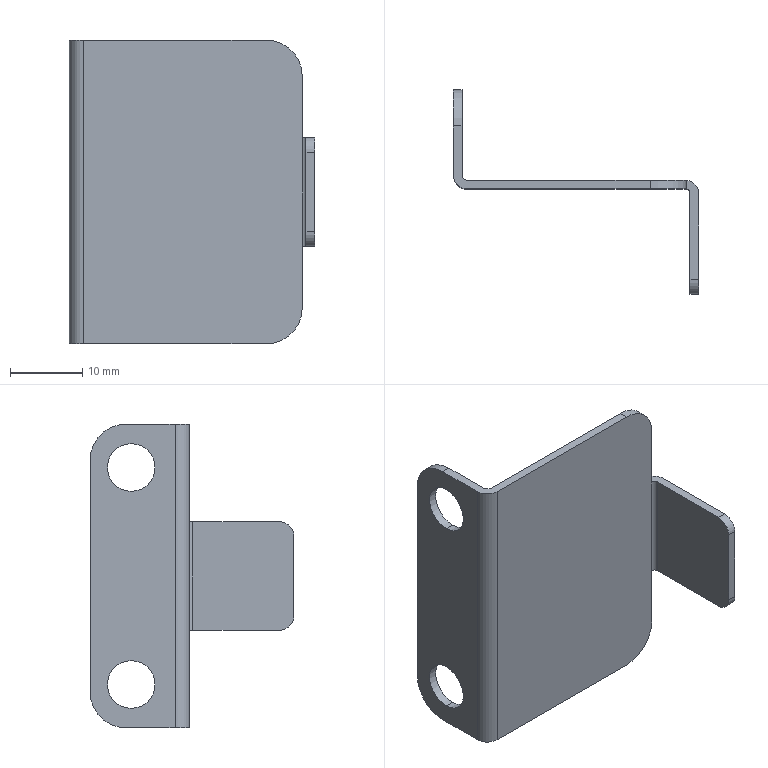Part | SolidWorks | features BaseBody 1 | 1 solid | 28 faces | box 33.9 x 28.2 x 42 mm | volume 2397 mm3 | cylinder 14 | plane 14 | commonest cylinder face diameters 6.6 x4 10 x4 4 x2 1 x1 1.473 x1 3.4 x1
STEP:
#1=CARTESIAN_POINT('',(0.,6.8,0.7));
#2=VERTEX_POINT('',#1);
#3=CARTESIAN_POINT('',(0.,6.8,7.3));
#4=VERTEX_POINT('',#3);
#5=CARTESIAN_POINT('',(0.,6.8,4.));
#6=DIRECTION('',(-1.,0.,0.));
#7=DIRECTION('',(0.,0.,1.));
#8=AXIS2_PLACEMENT_3D('',#5,#6,#7);
#9=CIRCLE('',#8,3.3);
#10=EDGE_CURVE('',#2,#4,#9,.T.);
#11=ORIENTED_EDGE('',*,*,#10,.F.);
#12=CARTESIAN_POINT('',(-1.2,6.8,0.7));
#13=VERTEX_POINT('',#12);
#14=CARTESIAN_POINT('',(-1.2,6.8,0.7));
#15=DIRECTION('',(-1.,0.,0.));
#16=VECTOR('',#15,1000.);
#17=LINE('',#14,#16);
#18=EDGE_CURVE('',#2,#13,#17,.T.);
#19=ORIENTED_EDGE('',*,*,#18,.T.);
#20=CARTESIAN_POINT('',(-1.2,6.8,7.3));
#21=VERTEX_POINT('',#20);
#22=CARTESIAN_POINT('',(-1.2,6.8,4.));
#23=DIRECTION('',(-1.,0.,0.));
#24=DIRECTION('',(0.,0.,1.));
#25=AXIS2_PLACEMENT_3D('',#22,#23,#24);
#26=CIRCLE('',#25,3.3);
#27=EDGE_CURVE('',#13,#21,#26,.T.);
#28=ORIENTED_EDGE('',*,*,#27,.T.);
#29=CARTESIAN_POINT('',(-1.2,6.8,7.3));
#30=DIRECTION('',(-1.,0.,0.));
#31=VECTOR('',#30,1000.);
#32=LINE('',#29,#31);
#33=EDGE_CURVE('',#4,#21,#32,.T.);
#34=ORIENTED_EDGE('',*,*,#33,.F.);
#35=EDGE_LOOP('',(#11,#19,#28,#34));
#36=FACE_OUTER_BOUND('',#35,.T.);
#37=CARTESIAN_POINT('',(-1.2,6.8,4.));
#38=DIRECTION('',(-1.,0.,0.));
#39=DIRECTION('',(0.,0.,1.));
#40=AXIS2_PLACEMENT_3D('',#37,#38,#39);
#41=CYLINDRICAL_SURFACE('',#40,3.3);
#42=ADVANCED_FACE('',(#36),#41,.F.);
#43=CARTESIAN_POINT('',(0.,6.8,-29.3));
#44=VERTEX_POINT('',#43);
#45=CARTESIAN_POINT('',(0.,6.8,-22.7));
#46=VERTEX_POINT('',#45);
#47=CARTESIAN_POINT('',(0.,6.8,-26.));
#48=DIRECTION('',(-1.,0.,0.));
#49=DIRECTION('',(0.,0.,1.));
#50=AXIS2_PLACEMENT_3D('',#47,#48,#49);
#51=CIRCLE('',#50,3.3);
#52=EDGE_CURVE('',#44,#46,#51,.T.);
#53=ORIENTED_EDGE('',*,*,#52,.F.);
#54=CARTESIAN_POINT('',(-1.2,6.8,-29.3));
#55=VERTEX_POINT('',#54);
#56=CARTESIAN_POINT('',(-1.2,6.8,-29.3));
#57=DIRECTION('',(-1.,0.,0.));
#58=VECTOR('',#57,1000.);
#59=LINE('',#56,#58);
#60=EDGE_CURVE('',#44,#55,#59,.T.);
#61=ORIENTED_EDGE('',*,*,#60,.T.);
#62=CARTESIAN_POINT('',(-1.2,6.8,-22.7));
#63=VERTEX_POINT('',#62);
#64=CARTESIAN_POINT('',(-1.2,6.8,-26.));
#65=DIRECTION('',(-1.,0.,0.));
#66=DIRECTION('',(0.,0.,1.));
#67=AXIS2_PLACEMENT_3D('',#64,#65,#66);
#68=CIRCLE('',#67,3.3);
#69=EDGE_CURVE('',#55,#63,#68,.T.);
#70=ORIENTED_EDGE('',*,*,#69,.T.);
#71=CARTESIAN_POINT('',(-1.2,6.8,-22.7));
#72=DIRECTION('',(-1.,0.,0.));
#73=VECTOR('',#72,1000.);
#74=LINE('',#71,#73);
#75=EDGE_CURVE('',#46,#63,#74,.T.);
#76=ORIENTED_EDGE('',*,*,#75,.F.);
#77=EDGE_LOOP('',(#53,#61,#70,#76));
#78=FACE_OUTER_BOUND('',#77,.T.);
#79=CARTESIAN_POINT('',(-1.2,6.8,-26.));
#80=DIRECTION('',(-1.,0.,0.));
#81=DIRECTION('',(0.,0.,1.));
#82=AXIS2_PLACEMENT_3D('',#79,#80,#81);
#83=CYLINDRICAL_SURFACE('',#82,3.3);
#84=ADVANCED_FACE('',(#78),#83,.F.);
#85=CARTESIAN_POINT('',(26.,-1.2,10.));
#86=VERTEX_POINT('',#85);
#87=CARTESIAN_POINT('',(31.,-1.2,5.));
#88=VERTEX_POINT('',#87);
#89=CARTESIAN_POINT('',(26.,-1.2,5.));
#90=DIRECTION('',(0.,1.,0.));
#91=DIRECTION('',(0.,0.,-1.));
#92=AXIS2_PLACEMENT_3D('',#89,#90,#91);
#93=CIRCLE('',#92,5.);
#94=EDGE_CURVE('',#86,#88,#93,.T.);
#95=ORIENTED_EDGE('',*,*,#94,.F.);
#96=CARTESIAN_POINT('',(0.7366,-1.2,10.));
#97=VERTEX_POINT('',#96);
#98=CARTESIAN_POINT('',(0.,-1.2,10.));
#99=DIRECTION('',(1.,0.,0.));
#100=VECTOR('',#99,1000.);
#101=LINE('',#98,#100);
#102=EDGE_CURVE('',#97,#86,#101,.T.);
#103=ORIENTED_EDGE('',*,*,#102,.F.);
#104=CARTESIAN_POINT('',(0.7366,-1.2,-32.));
#105=VERTEX_POINT('',#104);
#106=CARTESIAN_POINT('',(0.7366,-1.2,10.));
#107=DIRECTION('',(0.,0.,1.));
#108=VECTOR('',#107,1000.);
#109=LINE('',#106,#108);
#110=EDGE_CURVE('',#105,#97,#109,.T.);
#111=ORIENTED_EDGE('',*,*,#110,.F.);
#112=CARTESIAN_POINT('',(26.,-1.2,-32.));
#113=VERTEX_POINT('',#112);
#114=CARTESIAN_POINT('',(0.,-1.2,-32.));
#115=DIRECTION('',(-1.,0.,0.));
#116=VECTOR('',#115,1000.);
#117=LINE('',#114,#116);
#118=EDGE_CURVE('',#113,#105,#117,.T.);
#119=ORIENTED_EDGE('',*,*,#118,.F.);
#120=CARTESIAN_POINT('',(31.,-1.2,-27.));
#121=VERTEX_POINT('',#120);
#122=CARTESIAN_POINT('',(26.,-1.2,-27.));
#123=DIRECTION('',(0.,1.,0.));
#124=DIRECTION('',(0.,0.,-1.));
#125=AXIS2_PLACEMENT_3D('',#122,#123,#124);
#126=CIRCLE('',#125,5.);
#127=EDGE_CURVE('',#121,#113,#126,.T.);
#128=ORIENTED_EDGE('',*,*,#127,.F.);
#129=CARTESIAN_POINT('',(31.,-1.2,-18.5));
#130=VERTEX_POINT('',#129);
#131=CARTESIAN_POINT('',(31.,-1.2,10.));
#132=DIRECTION('',(0.,0.,-1.));
#133=VECTOR('',#132,1000.);
#134=LINE('',#131,#133);
#135=EDGE_CURVE('',#130,#121,#134,.T.);
#136=ORIENTED_EDGE('',*,*,#135,.F.);
#137=CARTESIAN_POINT('',(31.,-1.2,-3.5));
#138=VERTEX_POINT('',#137);
#139=CARTESIAN_POINT('',(31.,-1.2,10.));
#140=DIRECTION('',(0.,0.,-1.));
#141=VECTOR('',#140,1000.);
#142=LINE('',#139,#141);
#143=EDGE_CURVE('',#138,#130,#142,.T.);
#144=ORIENTED_EDGE('',*,*,#143,.F.);
#145=CARTESIAN_POINT('',(31.,-1.2,10.));
#146=DIRECTION('',(0.,0.,-1.));
#147=VECTOR('',#146,1000.);
#148=LINE('',#145,#147);
#149=EDGE_CURVE('',#88,#138,#148,.T.);
#150=ORIENTED_EDGE('',*,*,#149,.F.);
#151=EDGE_LOOP('',(#95,#103,#111,#119,#128,#136,#144,#150));
#152=FACE_OUTER_BOUND('',#151,.T.);
#153=CARTESIAN_POINT('',(0.,-1.2,10.));
#154=DIRECTION('',(0.,1.,0.));
#155=DIRECTION('',(0.,0.,1.));
#156=AXIS2_PLACEMENT_3D('',#153,#154,#155);
#157=PLANE('',#156);
#158=ADVANCED_FACE('',(#152),#157,.F.);
#159=ORIENTED_EDGE('',*,*,#149,.T.);
#160=CARTESIAN_POINT('',(31.,0.,-3.5));
#161=VERTEX_POINT('',#160);
#162=CARTESIAN_POINT('',(31.,-1.7,-3.5));
#163=DIRECTION('',(0.,1.,0.));
#164=VECTOR('',#163,1000.);
#165=LINE('',#162,#164);
#166=EDGE_CURVE('',#138,#161,#165,.T.);
#167=ORIENTED_EDGE('',*,*,#166,.T.);
#168=CARTESIAN_POINT('',(31.,0.,5.));
#169=VERTEX_POINT('',#168);
#170=CARTESIAN_POINT('',(31.,0.,10.));
#171=DIRECTION('',(0.,0.,1.));
#172=VECTOR('',#171,1000.);
#173=LINE('',#170,#172);
#174=EDGE_CURVE('',#161,#169,#173,.T.);
#175=ORIENTED_EDGE('',*,*,#174,.T.);
#176=CARTESIAN_POINT('',(31.,0.,5.));
#177=DIRECTION('',(0.,-1.,0.));
#178=VECTOR('',#177,1000.);
#179=LINE('',#176,#178);
#180=EDGE_CURVE('',#169,#88,#179,.T.);
#181=ORIENTED_EDGE('',*,*,#180,.T.);
#182=EDGE_LOOP('',(#159,#167,#175,#181));
#183=FACE_OUTER_BOUND('',#182,.T.);
#184=CARTESIAN_POINT('',(31.,0.,10.));
#185=DIRECTION('',(1.,0.,0.));
#186=DIRECTION('',(0.,0.,-1.));
#187=AXIS2_PLACEMENT_3D('',#184,#185,#186);
#188=PLANE('',#187);
#189=ADVANCED_FACE('',(#183),#188,.T.);
#190=ORIENTED_EDGE('',*,*,#94,.T.);
#191=ORIENTED_EDGE('',*,*,#180,.F.);
#192=CARTESIAN_POINT('',(26.,0.,10.));
#193=VERTEX_POINT('',#192);
#194=CARTESIAN_POINT('',(26.,0.,5.));
#195=DIRECTION('',(0.,-1.,0.));
#196=DIRECTION('',(0.,0.,-1.));
#197=AXIS2_PLACEMENT_3D('',#194,#195,#196);
#198=CIRCLE('',#197,5.);
#199=EDGE_CURVE('',#169,#193,#198,.T.);
#200=ORIENTED_EDGE('',*,*,#199,.T.);
#201=CARTESIAN_POINT('',(26.,0.,10.));
#202=DIRECTION('',(0.,-1.,0.));
#203=VECTOR('',#202,1000.);
#204=LINE('',#201,#203);
#205=EDGE_CURVE('',#193,#86,#204,.T.);
#206=ORIENTED_EDGE('',*,*,#205,.T.);
#207=EDGE_LOOP('',(#190,#191,#200,#206));
#208=FACE_OUTER_BOUND('',#207,.T.);
#209=CARTESIAN_POINT('',(26.,0.,5.));
#210=DIRECTION('',(0.,-1.,0.));
#211=DIRECTION('',(0.,0.,-1.));
#212=AXIS2_PLACEMENT_3D('',#209,#210,#211);
#213=CYLINDRICAL_SURFACE('',#212,5.);
#214=ADVANCED_FACE('',(#208),#213,.T.);
#215=CARTESIAN_POINT('',(0.7366,0.,10.));
#216=VERTEX_POINT('',#215);
#217=CARTESIAN_POINT('',(-1.2,0.,10.));
#218=DIRECTION('',(-1.,0.,0.));
#219=VECTOR('',#218,1000.);
#220=LINE('',#217,#219);
#221=EDGE_CURVE('',#193,#216,#220,.T.);
#222=ORIENTED_EDGE('',*,*,#221,.T.);
#223=CARTESIAN_POINT('',(0.,0.7366,10.));
#224=VERTEX_POINT('',#223);
#225=CARTESIAN_POINT('',(0.7366,0.7366,10.));
#226=DIRECTION('',(0.,0.,-1.));
#227=DIRECTION('',(-1.,0.,0.));
#228=AXIS2_PLACEMENT_3D('',#225,#226,#227);
#229=CIRCLE('',#228,0.7366);
#230=EDGE_CURVE('',#216,#224,#229,.T.);
#231=ORIENTED_EDGE('',*,*,#230,.T.);
#232=CARTESIAN_POINT('',(0.,7.5,10.));
#233=VERTEX_POINT('',#232);
#234=CARTESIAN_POINT('',(0.,0.7366,10.));
#235=DIRECTION('',(0.,-1.,0.));
#236=VECTOR('',#235,1000.);
#237=LINE('',#234,#236);
#238=EDGE_CURVE('',#233,#224,#237,.T.);
#239=ORIENTED_EDGE('',*,*,#238,.F.);
#240=CARTESIAN_POINT('',(-1.2,7.5,10.));
#241=VERTEX_POINT('',#240);
#242=CARTESIAN_POINT('',(0.7366,7.5,10.));
#243=DIRECTION('',(1.,0.,0.));
#244=VECTOR('',#243,1000.);
#245=LINE('',#242,#244);
#246=EDGE_CURVE('',#241,#233,#245,.T.);
#247=ORIENTED_EDGE('',*,*,#246,.F.);
#248=CARTESIAN_POINT('',(-1.2,0.7366,10.));
#249=VERTEX_POINT('',#248);
#250=CARTESIAN_POINT('',(-1.2,12.5,10.));
#251=DIRECTION('',(0.,-1.,0.));
#252=VECTOR('',#251,1000.);
#253=LINE('',#250,#252);
#254=EDGE_CURVE('',#241,#249,#253,.T.);
#255=ORIENTED_EDGE('',*,*,#254,.T.);
#256=CARTESIAN_POINT('',(0.7366,0.7366,10.));
#257=DIRECTION('',(0.,0.,-1.));
#258=DIRECTION('',(-1.,0.,0.));
#259=AXIS2_PLACEMENT_3D('',#256,#257,#258);
#260=CIRCLE('',#259,1.937);
#261=EDGE_CURVE('',#97,#249,#260,.T.);
#262=ORIENTED_EDGE('',*,*,#261,.F.);
#263=ORIENTED_EDGE('',*,*,#102,.T.);
#264=ORIENTED_EDGE('',*,*,#205,.F.);
#265=EDGE_LOOP('',(#222,#231,#239,#247,#255,#262,#263,#264));
#266=FACE_OUTER_BOUND('',#265,.T.);
#267=CARTESIAN_POINT('',(-1.2,0.7366,10.));
#268=DIRECTION('',(0.,0.,1.));
#269=DIRECTION('',(1.,0.,0.));
#270=AXIS2_PLACEMENT_3D('',#267,#268,#269);
#271=PLANE('',#270);
#272=ADVANCED_FACE('',(#266),#271,.T.);
#273=ORIENTED_EDGE('',*,*,#110,.T.);
#274=ORIENTED_EDGE('',*,*,#261,.T.);
#275=CARTESIAN_POINT('',(-1.2,0.7366,-32.));
#276=VERTEX_POINT('',#275);
#277=CARTESIAN_POINT('',(-1.2,0.7366,10.));
#278=DIRECTION('',(0.,0.,-1.));
#279=VECTOR('',#278,1000.);
#280=LINE('',#277,#279);
#281=EDGE_CURVE('',#249,#276,#280,.T.);
#282=ORIENTED_EDGE('',*,*,#281,.T.);
#283=CARTESIAN_POINT('',(0.7366,0.7366,-32.));
#284=DIRECTION('',(0.,0.,1.));
#285=DIRECTION('',(-1.,0.,0.));
#286=AXIS2_PLACEMENT_3D('',#283,#284,#285);
#287=CIRCLE('',#286,1.937);
#288=EDGE_CURVE('',#276,#105,#287,.T.);
#289=ORIENTED_EDGE('',*,*,#288,.T.);
#290=EDGE_LOOP('',(#273,#274,#282,#289));
#291=FACE_OUTER_BOUND('',#290,.T.);
#292=CARTESIAN_POINT('',(0.7366,0.7366,10.));
#293=DIRECTION('',(0.,0.,-1.));
#294=DIRECTION('',(-1.,0.,0.));
#295=AXIS2_PLACEMENT_3D('',#292,#293,#294);
#296=CYLINDRICAL_SURFACE('',#295,1.937);
#297=ADVANCED_FACE('',(#291),#296,.T.);
#298=ORIENTED_EDGE('',*,*,#118,.T.);
#299=ORIENTED_EDGE('',*,*,#288,.F.);
#300=CARTESIAN_POINT('',(-1.2,7.5,-32.));
#301=VERTEX_POINT('',#300);
#302=CARTESIAN_POINT('',(-1.2,12.5,-32.));
#303=DIRECTION('',(0.,1.,0.));
#304=VECTOR('',#303,1000.);
#305=LINE('',#302,#304);
#306=EDGE_CURVE('',#276,#301,#305,.T.);
#307=ORIENTED_EDGE('',*,*,#306,.T.);
#308=CARTESIAN_POINT('',(0.,7.5,-32.));
#309=VERTEX_POINT('',#308);
#310=CARTESIAN_POINT('',(0.7366,7.5,-32.));
#311=DIRECTION('',(-1.,0.,0.));
#312=VECTOR('',#311,1000.);
#313=LINE('',#310,#312);
#314=EDGE_CURVE('',#309,#301,#313,.T.);
#315=ORIENTED_EDGE('',*,*,#314,.F.);
#316=CARTESIAN_POINT('',(0.,0.7366,-32.));
#317=VERTEX_POINT('',#316);
#318=CARTESIAN_POINT('',(0.,-1.2,-32.));
#319=DIRECTION('',(0.,-1.,0.));
#320=VECTOR('',#319,1000.);
#321=LINE('',#318,#320);
#322=EDGE_CURVE('',#309,#317,#321,.T.);
#323=ORIENTED_EDGE('',*,*,#322,.T.);
#324=CARTESIAN_POINT('',(0.7366,0.,-32.));
#325=VERTEX_POINT('',#324);
#326=CARTESIAN_POINT('',(0.7366,0.7366,-32.));
#327=DIRECTION('',(0.,0.,1.));
#328=DIRECTION('',(-1.,0.,0.));
#329=AXIS2_PLACEMENT_3D('',#326,#327,#328);
#330=CIRCLE('',#329,0.7366);
#331=EDGE_CURVE('',#317,#325,#330,.T.);
#332=ORIENTED_EDGE('',*,*,#331,.T.);
#333=CARTESIAN_POINT('',(26.,0.,-32.));
#334=VERTEX_POINT('',#333);
#335=CARTESIAN_POINT('',(0.7366,0.,-32.));
#336=DIRECTION('',(1.,0.,0.));
#337=VECTOR('',#336,1000.);
#338=LINE('',#335,#337);
#339=EDGE_CURVE('',#325,#334,#338,.T.);
#340=ORIENTED_EDGE('',*,*,#339,.T.);
#341=CARTESIAN_POINT('',(26.,0.7366,-32.));
#342=DIRECTION('',(0.,-1.,0.));
#343=VECTOR('',#342,1000.);
#344=LINE('',#341,#343);
#345=EDGE_CURVE('',#334,#113,#344,.T.);
#346=ORIENTED_EDGE('',*,*,#345,.T.);
#347=EDGE_LOOP('',(#298,#299,#307,#315,#323,#332,#340,#346));
#348=FACE_OUTER_BOUND('',#347,.T.);
#349=CARTESIAN_POINT('',(0.7366,0.7366,-32.));
#350=DIRECTION('',(0.,0.,-1.));
#351=DIRECTION('',(-1.,0.,0.));
#352=AXIS2_PLACEMENT_3D('',#349,#350,#351);
#353=PLANE('',#352);
#354=ADVANCED_FACE('',(#348),#353,.T.);
#355=ORIENTED_EDGE('',*,*,#127,.T.);
#356=ORIENTED_EDGE('',*,*,#345,.F.);
#357=CARTESIAN_POINT('',(31.,0.,-27.));
#358=VERTEX_POINT('',#357);
#359=CARTESIAN_POINT('',(26.,0.,-27.));
#360=DIRECTION('',(0.,-1.,0.));
#361=DIRECTION('',(0.,0.,-1.));
#362=AXIS2_PLACEMENT_3D('',#359,#360,#361);
#363=CIRCLE('',#362,5.);
#364=EDGE_CURVE('',#334,#358,#363,.T.);
#365=ORIENTED_EDGE('',*,*,#364,.T.);
#366=CARTESIAN_POINT('',(31.,0.7366,-27.));
#367=DIRECTION('',(0.,-1.,0.));
#368=VECTOR('',#367,1000.);
#369=LINE('',#366,#368);
#370=EDGE_CURVE('',#358,#121,#369,.T.);
#371=ORIENTED_EDGE('',*,*,#370,.T.);
#372=EDGE_LOOP('',(#355,#356,#365,#371));
#373=FACE_OUTER_BOUND('',#372,.T.);
#374=CARTESIAN_POINT('',(26.,0.7366,-27.));
#375=DIRECTION('',(0.,-1.,0.));
#376=DIRECTION('',(0.,0.,-1.));
#377=AXIS2_PLACEMENT_3D('',#374,#375,#376);
#378=CYLINDRICAL_SURFACE('',#377,5.);
#379=ADVANCED_FACE('',(#373),#378,.T.);
#380=CARTESIAN_POINT('',(31.,0.,-18.5));
#381=VERTEX_POINT('',#380);
#382=CARTESIAN_POINT('',(31.,0.,10.));
#383=DIRECTION('',(0.,0.,1.));
#384=VECTOR('',#383,1000.);
#385=LINE('',#382,#384);
#386=EDGE_CURVE('',#358,#381,#385,.T.);
#387=ORIENTED_EDGE('',*,*,#386,.T.);
#388=CARTESIAN_POINT('',(31.,-1.7,-18.5));
#389=DIRECTION('',(0.,1.,0.));
#390=VECTOR('',#389,1000.);
#391=LINE('',#388,#390);
#392=EDGE_CURVE('',#130,#381,#391,.T.);
#393=ORIENTED_EDGE('',*,*,#392,.F.);
#394=ORIENTED_EDGE('',*,*,#135,.T.);
#395=ORIENTED_EDGE('',*,*,#370,.F.);
#396=EDGE_LOOP('',(#387,#393,#394,#395));
#397=FACE_OUTER_BOUND('',#396,.T.);
#398=CARTESIAN_POINT('',(31.,0.,10.));
#399=DIRECTION('',(1.,0.,0.));
#400=DIRECTION('',(0.,0.,-1.));
#401=AXIS2_PLACEMENT_3D('',#398,#399,#400);
#402=PLANE('',#401);
#403=ADVANCED_FACE('',(#397),#402,.T.);
#404=CARTESIAN_POINT('',(31.5,-1.7,-18.5));
#405=VERTEX_POINT('',#404);
#406=CARTESIAN_POINT('',(31.,-1.7,-18.5));
#407=DIRECTION('',(0.,0.,1.));
#408=DIRECTION('',(1.,0.,0.));
#409=AXIS2_PLACEMENT_3D('',#406,#407,#408);
#410=CIRCLE('',#409,0.5);
#411=EDGE_CURVE('',#405,#130,#410,.T.);
#412=ORIENTED_EDGE('',*,*,#411,.F.);
#413=CARTESIAN_POINT('',(31.5,-1.7,-3.5));
#414=VERTEX_POINT('',#413);
#415=CARTESIAN_POINT('',(31.5,-1.7,-3.5));
#416=DIRECTION('',(0.,0.,-1.));
#417=VECTOR('',#416,1000.);
#418=LINE('',#415,#417);
#419=EDGE_CURVE('',#414,#405,#418,.T.);
#420=ORIENTED_EDGE('',*,*,#419,.F.);
#421=CARTESIAN_POINT('',(31.,-1.7,-3.5));
#422=DIRECTION('',(0.,0.,1.));
#423=DIRECTION('',(1.,0.,0.));
#424=AXIS2_PLACEMENT_3D('',#421,#422,#423);
#425=CIRCLE('',#424,0.5);
#426=EDGE_CURVE('',#414,#138,#425,.T.);
#427=ORIENTED_EDGE('',*,*,#426,.T.);
#428=ORIENTED_EDGE('',*,*,#143,.T.);
#429=EDGE_LOOP('',(#412,#420,#427,#428));
#430=FACE_OUTER_BOUND('',#429,.T.);
#431=CARTESIAN_POINT('',(31.,-1.7,-3.5));
#432=DIRECTION('',(0.,0.,1.));
#433=DIRECTION('',(1.,0.,0.));
#434=AXIS2_PLACEMENT_3D('',#431,#432,#433);
#435=CYLINDRICAL_SURFACE('',#434,0.5);
#436=ADVANCED_FACE('',(#430),#435,.F.);
#437=ORIENTED_EDGE('',*,*,#339,.F.);
#438=CARTESIAN_POINT('',(0.7366,0.,10.));
#439=DIRECTION('',(0.,0.,1.));
#440=VECTOR('',#439,1000.);
#441=LINE('',#438,#440);
#442=EDGE_CURVE('',#325,#216,#441,.T.);
#443=ORIENTED_EDGE('',*,*,#442,.T.);
#444=ORIENTED_EDGE('',*,*,#221,.F.);
#445=ORIENTED_EDGE('',*,*,#199,.F.);
#446=ORIENTED_EDGE('',*,*,#174,.F.);
#447=CARTESIAN_POINT('',(31.,0.,10.));
#448=DIRECTION('',(0.,0.,-1.));
#449=VECTOR('',#448,1000.);
#450=LINE('',#447,#449);
#451=EDGE_CURVE('',#161,#381,#450,.T.);
#452=ORIENTED_EDGE('',*,*,#451,.T.);
#453=ORIENTED_EDGE('',*,*,#386,.F.);
#454=ORIENTED_EDGE('',*,*,#364,.F.);
#455=EDGE_LOOP('',(#437,#443,#444,#445,#446,#452,#453,#454));
#456=FACE_OUTER_BOUND('',#455,.T.);
#457=CARTESIAN_POINT('',(0.,0.,10.));
#458=DIRECTION('',(0.,1.,0.));
#459=DIRECTION('',(0.,0.,1.));
#460=AXIS2_PLACEMENT_3D('',#457,#458,#459);
#461=PLANE('',#460);
#462=ADVANCED_FACE('',(#456),#461,.T.);
#463=CARTESIAN_POINT('',(-1.2,12.5,5.));
#464=VERTEX_POINT('',#463);
#465=CARTESIAN_POINT('',(-1.2,7.5,5.));
#466=DIRECTION('',(1.,0.,0.));
#467=DIRECTION('',(0.,0.,1.));
#468=AXIS2_PLACEMENT_3D('',#465,#466,#467);
#469=CIRCLE('',#468,5.);
#470=EDGE_CURVE('',#464,#241,#469,.T.);
#471=ORIENTED_EDGE('',*,*,#470,.F.);
#472=CARTESIAN_POINT('',(-1.2,12.5,-27.));
#473=VERTEX_POINT('',#472);
#474=CARTESIAN_POINT('',(-1.2,12.5,10.));
#475=DIRECTION('',(0.,0.,1.));
#476=VECTOR('',#475,1000.);
#477=LINE('',#474,#476);
#478=EDGE_CURVE('',#473,#464,#477,.T.);
#479=ORIENTED_EDGE('',*,*,#478,.F.);
#480=CARTESIAN_POINT('',(-1.2,7.5,-27.));
#481=DIRECTION('',(1.,0.,0.));
#482=DIRECTION('',(0.,0.,-1.));
#483=AXIS2_PLACEMENT_3D('',#480,#481,#482);
#484=CIRCLE('',#483,5.);
#485=EDGE_CURVE('',#301,#473,#484,.T.);
#486=ORIENTED_EDGE('',*,*,#485,.F.);
#487=ORIENTED_EDGE('',*,*,#306,.F.);
#488=ORIENTED_EDGE('',*,*,#281,.F.);
#489=ORIENTED_EDGE('',*,*,#254,.F.);
#490=EDGE_LOOP('',(#471,#479,#486,#487,#488,#489));
#491=FACE_OUTER_BOUND('',#490,.T.);
#492=CARTESIAN_POINT('',(-1.2,6.8,4.));
#493=DIRECTION('',(-1.,0.,0.));
#494=DIRECTION('',(0.,0.,1.));
#495=AXIS2_PLACEMENT_3D('',#492,#493,#494);
#496=CIRCLE('',#495,3.3);
#497=EDGE_CURVE('',#21,#13,#496,.T.);
#498=ORIENTED_EDGE('',*,*,#497,.F.);
#499=ORIENTED_EDGE('',*,*,#27,.F.);
#500=EDGE_LOOP('',(#498,#499));
#501=FACE_BOUND('',#500,.T.);
#502=CARTESIAN_POINT('',(-1.2,6.8,-26.));
#503=DIRECTION('',(-1.,0.,0.));
#504=DIRECTION('',(0.,0.,1.));
#505=AXIS2_PLACEMENT_3D('',#502,#503,#504);
#506=CIRCLE('',#505,3.3);
#507=EDGE_CURVE('',#63,#55,#506,.T.);
#508=ORIENTED_EDGE('',*,*,#507,.F.);
#509=ORIENTED_EDGE('',*,*,#69,.F.);
#510=EDGE_LOOP('',(#508,#509));
#511=FACE_BOUND('',#510,.T.);
#512=CARTESIAN_POINT('',(-1.2,12.5,10.));
#513=DIRECTION('',(1.,0.,0.));
#514=DIRECTION('',(0.,1.,0.));
#515=AXIS2_PLACEMENT_3D('',#512,#513,#514);
#516=PLANE('',#515);
#517=ADVANCED_FACE('',(#491,#501,#511),#516,.F.);
#518=CARTESIAN_POINT('',(31.5,-13.7,-18.5));
#519=VERTEX_POINT('',#518);
#520=CARTESIAN_POINT('',(31.5,0.,-18.5));
#521=DIRECTION('',(0.,-1.,0.));
#522=VECTOR('',#521,1000.);
#523=LINE('',#520,#522);
#524=EDGE_CURVE('',#405,#519,#523,.T.);
#525=ORIENTED_EDGE('',*,*,#524,.T.);
#526=CARTESIAN_POINT('',(31.5,-15.7,-16.5));
#527=VERTEX_POINT('',#526);
#528=CARTESIAN_POINT('',(31.5,-13.7,-16.5));
#529=DIRECTION('',(-1.,0.,0.));
#530=DIRECTION('',(0.,-1.,0.));
#531=AXIS2_PLACEMENT_3D('',#528,#529,#530);
#532=CIRCLE('',#531,2.);
#533=EDGE_CURVE('',#519,#527,#532,.T.);
#534=ORIENTED_EDGE('',*,*,#533,.T.);
#535=CARTESIAN_POINT('',(31.5,-15.7,-5.5));
#536=VERTEX_POINT('',#535);
#537=CARTESIAN_POINT('',(31.5,-15.7,0.));
#538=DIRECTION('',(0.,0.,1.));
#539=VECTOR('',#538,1000.);
#540=LINE('',#537,#539);
#541=EDGE_CURVE('',#527,#536,#540,.T.);
#542=ORIENTED_EDGE('',*,*,#541,.T.);
#543=CARTESIAN_POINT('',(31.5,-13.7,-3.5));
#544=VERTEX_POINT('',#543);
#545=CARTESIAN_POINT('',(31.5,-13.7,-5.5));
#546=DIRECTION('',(-1.,0.,0.));
#547=DIRECTION('',(0.,-1.,0.));
#548=AXIS2_PLACEMENT_3D('',#545,#546,#547);
#549=CIRCLE('',#548,2.);
#550=EDGE_CURVE('',#536,#544,#549,.T.);
#551=ORIENTED_EDGE('',*,*,#550,.T.);
#552=CARTESIAN_POINT('',(31.5,0.,-3.5));
#553=DIRECTION('',(0.,1.,0.));
#554=VECTOR('',#553,1000.);
#555=LINE('',#552,#554);
#556=EDGE_CURVE('',#544,#414,#555,.T.);
#557=ORIENTED_EDGE('',*,*,#556,.T.);
#558=ORIENTED_EDGE('',*,*,#419,.T.);
#559=EDGE_LOOP('',(#525,#534,#542,#551,#557,#558));
#560=FACE_OUTER_BOUND('',#559,.T.);
#561=CARTESIAN_POINT('',(31.5,0.,0.));
#562=DIRECTION('',(-1.,0.,0.));
#563=DIRECTION('',(0.,-1.,0.));
#564=AXIS2_PLACEMENT_3D('',#561,#562,#563);
#565=PLANE('',#564);
#566=ADVANCED_FACE('',(#560),#565,.T.);
#567=ORIENTED_EDGE('',*,*,#331,.F.);
#568=CARTESIAN_POINT('',(0.,0.7366,10.));
#569=DIRECTION('',(0.,0.,-1.));
#570=VECTOR('',#569,1000.);
#571=LINE('',#568,#570);
#572=EDGE_CURVE('',#224,#317,#571,.T.);
#573=ORIENTED_EDGE('',*,*,#572,.F.);
#574=ORIENTED_EDGE('',*,*,#230,.F.);
#575=ORIENTED_EDGE('',*,*,#442,.F.);
#576=EDGE_LOOP('',(#567,#573,#574,#575));
#577=FACE_OUTER_BOUND('',#576,.T.);
#578=CARTESIAN_POINT('',(0.7366,0.7366,10.));
#579=DIRECTION('',(0.,0.,-1.));
#580=DIRECTION('',(-1.,0.,0.));
#581=AXIS2_PLACEMENT_3D('',#578,#579,#580);
#582=CYLINDRICAL_SURFACE('',#581,0.7366);
#583=ADVANCED_FACE('',(#577),#582,.F.);
#584=CARTESIAN_POINT('',(32.7,-1.7,-3.5));
#585=VERTEX_POINT('',#584);
#586=CARTESIAN_POINT('',(32.7,-1.7,-18.5));
#587=VERTEX_POINT('',#586);
#588=CARTESIAN_POINT('',(32.7,-1.7,-3.5));
#589=DIRECTION('',(0.,0.,-1.));
#590=VECTOR('',#589,1000.);
#591=LINE('',#588,#590);
#592=EDGE_CURVE('',#585,#587,#591,.T.);
#593=ORIENTED_EDGE('',*,*,#592,.T.);
#594=CARTESIAN_POINT('',(31.,-1.7,-18.5));
#595=DIRECTION('',(0.,0.,1.));
#596=DIRECTION('',(1.,0.,0.));
#597=AXIS2_PLACEMENT_3D('',#594,#595,#596);
#598=CIRCLE('',#597,1.7);
#599=EDGE_CURVE('',#587,#381,#598,.T.);
#600=ORIENTED_EDGE('',*,*,#599,.T.);
#601=ORIENTED_EDGE('',*,*,#451,.F.);
#602=CARTESIAN_POINT('',(31.,-1.7,-3.5));
#603=DIRECTION('',(0.,0.,-1.));
#604=DIRECTION('',(1.,0.,0.));
#605=AXIS2_PLACEMENT_3D('',#602,#603,#604);
#606=CIRCLE('',#605,1.7);
#607=EDGE_CURVE('',#161,#585,#606,.T.);
#608=ORIENTED_EDGE('',*,*,#607,.T.);
#609=EDGE_LOOP('',(#593,#600,#601,#608));
#610=FACE_OUTER_BOUND('',#609,.T.);
#611=CARTESIAN_POINT('',(31.,-1.7,-3.5));
#612=DIRECTION('',(0.,0.,1.));
#613=DIRECTION('',(1.,0.,0.));
#614=AXIS2_PLACEMENT_3D('',#611,#612,#613);
#615=CYLINDRICAL_SURFACE('',#614,1.7);
#616=ADVANCED_FACE('',(#610),#615,.T.);
#617=CARTESIAN_POINT('',(0.,12.5,5.));
#618=VERTEX_POINT('',#617);
#619=CARTESIAN_POINT('',(0.,7.5,5.));
#620=DIRECTION('',(-1.,0.,0.));
#621=DIRECTION('',(0.,0.,1.));
#622=AXIS2_PLACEMENT_3D('',#619,#620,#621);
#623=CIRCLE('',#622,5.);
#624=EDGE_CURVE('',#233,#618,#623,.T.);
#625=ORIENTED_EDGE('',*,*,#624,.T.);
#626=CARTESIAN_POINT('',(-1.2,12.5,5.));
#627=DIRECTION('',(-1.,0.,0.));
#628=VECTOR('',#627,1000.);
#629=LINE('',#626,#628);
#630=EDGE_CURVE('',#618,#464,#629,.T.);
#631=ORIENTED_EDGE('',*,*,#630,.T.);
#632=ORIENTED_EDGE('',*,*,#470,.T.);
#633=ORIENTED_EDGE('',*,*,#246,.T.);
#634=EDGE_LOOP('',(#625,#631,#632,#633));
#635=FACE_OUTER_BOUND('',#634,.T.);
#636=CARTESIAN_POINT('',(-1.2,7.5,5.));
#637=DIRECTION('',(-1.,0.,0.));
#638=DIRECTION('',(0.,0.,1.));
#639=AXIS2_PLACEMENT_3D('',#636,#637,#638);
#640=CYLINDRICAL_SURFACE('',#639,5.);
#641=ADVANCED_FACE('',(#635),#640,.T.);
#642=CARTESIAN_POINT('',(0.,12.5,-27.));
#643=VERTEX_POINT('',#642);
#644=CARTESIAN_POINT('',(0.,12.5,10.));
#645=DIRECTION('',(0.,0.,-1.));
#646=VECTOR('',#645,1000.);
#647=LINE('',#644,#646);
#648=EDGE_CURVE('',#618,#643,#647,.T.);
#649=ORIENTED_EDGE('',*,*,#648,.T.);
#650=CARTESIAN_POINT('',(-1.2,12.5,-27.));
#651=DIRECTION('',(-1.,0.,0.));
#652=VECTOR('',#651,1000.);
#653=LINE('',#650,#652);
#654=EDGE_CURVE('',#643,#473,#653,.T.);
#655=ORIENTED_EDGE('',*,*,#654,.T.);
#656=ORIENTED_EDGE('',*,*,#478,.T.);
#657=ORIENTED_EDGE('',*,*,#630,.F.);
#658=EDGE_LOOP('',(#649,#655,#656,#657));
#659=FACE_OUTER_BOUND('',#658,.T.);
#660=CARTESIAN_POINT('',(-1.2,12.5,10.));
#661=DIRECTION('',(0.,1.,0.));
#662=DIRECTION('',(0.,0.,1.));
#663=AXIS2_PLACEMENT_3D('',#660,#661,#662);
#664=PLANE('',#663);
#665=ADVANCED_FACE('',(#659),#664,.T.);
#666=CARTESIAN_POINT('',(0.,7.5,-27.));
#667=DIRECTION('',(-1.,0.,0.));
#668=DIRECTION('',(0.,0.,-1.));
#669=AXIS2_PLACEMENT_3D('',#666,#667,#668);
#670=CIRCLE('',#669,5.);
#671=EDGE_CURVE('',#643,#309,#670,.T.);
#672=ORIENTED_EDGE('',*,*,#671,.T.);
#673=ORIENTED_EDGE('',*,*,#314,.T.);
#674=ORIENTED_EDGE('',*,*,#485,.T.);
#675=ORIENTED_EDGE('',*,*,#654,.F.);
#676=EDGE_LOOP('',(#672,#673,#674,#675));
#677=FACE_OUTER_BOUND('',#676,.T.);
#678=CARTESIAN_POINT('',(0.7366,7.5,-27.));
#679=DIRECTION('',(1.,0.,0.));
#680=DIRECTION('',(0.,0.,-1.));
#681=AXIS2_PLACEMENT_3D('',#678,#679,#680);
#682=CYLINDRICAL_SURFACE('',#681,5.);
#683=ADVANCED_FACE('',(#677),#682,.T.);
#684=ORIENTED_EDGE('',*,*,#18,.F.);
#685=CARTESIAN_POINT('',(0.,6.8,4.));
#686=DIRECTION('',(-1.,0.,0.));
#687=DIRECTION('',(0.,0.,1.));
#688=AXIS2_PLACEMENT_3D('',#685,#686,#687);
#689=CIRCLE('',#688,3.3);
#690=EDGE_CURVE('',#4,#2,#689,.T.);
#691=ORIENTED_EDGE('',*,*,#690,.F.);
#692=ORIENTED_EDGE('',*,*,#33,.T.);
#693=ORIENTED_EDGE('',*,*,#497,.T.);
#694=EDGE_LOOP('',(#684,#691,#692,#693));
#695=FACE_OUTER_BOUND('',#694,.T.);
#696=CARTESIAN_POINT('',(-1.2,6.8,4.));
#697=DIRECTION('',(-1.,0.,0.));
#698=DIRECTION('',(0.,0.,1.));
#699=AXIS2_PLACEMENT_3D('',#696,#697,#698);
#700=CYLINDRICAL_SURFACE('',#699,3.3);
#701=ADVANCED_FACE('',(#695),#700,.F.);
#702=ORIENTED_EDGE('',*,*,#60,.F.);
#703=CARTESIAN_POINT('',(0.,6.8,-26.));
#704=DIRECTION('',(-1.,0.,0.));
#705=DIRECTION('',(0.,0.,1.));
#706=AXIS2_PLACEMENT_3D('',#703,#704,#705);
#707=CIRCLE('',#706,3.3);
#708=EDGE_CURVE('',#46,#44,#707,.T.);
#709=ORIENTED_EDGE('',*,*,#708,.F.);
#710=ORIENTED_EDGE('',*,*,#75,.T.);
#711=ORIENTED_EDGE('',*,*,#507,.T.);
#712=EDGE_LOOP('',(#702,#709,#710,#711));
#713=FACE_OUTER_BOUND('',#712,.T.);
#714=CARTESIAN_POINT('',(-1.2,6.8,-26.));
#715=DIRECTION('',(-1.,0.,0.));
#716=DIRECTION('',(0.,0.,1.));
#717=AXIS2_PLACEMENT_3D('',#714,#715,#716);
#718=CYLINDRICAL_SURFACE('',#717,3.3);
#719=ADVANCED_FACE('',(#713),#718,.F.);
#720=ORIENTED_EDGE('',*,*,#533,.F.);
#721=CARTESIAN_POINT('',(32.7,-13.7,-18.5));
#722=VERTEX_POINT('',#721);
#723=CARTESIAN_POINT('',(32.7,-13.7,-18.5));
#724=DIRECTION('',(1.,0.,0.));
#725=VECTOR('',#724,1000.);
#726=LINE('',#723,#725);
#727=EDGE_CURVE('',#519,#722,#726,.T.);
#728=ORIENTED_EDGE('',*,*,#727,.T.);
#729=CARTESIAN_POINT('',(32.7,-15.7,-16.5));
#730=VERTEX_POINT('',#729);
#731=CARTESIAN_POINT('',(32.7,-13.7,-16.5));
#732=DIRECTION('',(-1.,0.,0.));
#733=DIRECTION('',(0.,-1.,0.));
#734=AXIS2_PLACEMENT_3D('',#731,#732,#733);
#735=CIRCLE('',#734,2.);
#736=EDGE_CURVE('',#722,#730,#735,.T.);
#737=ORIENTED_EDGE('',*,*,#736,.T.);
#738=CARTESIAN_POINT('',(32.7,-15.7,-16.5));
#739=DIRECTION('',(-1.,0.,0.));
#740=VECTOR('',#739,1000.);
#741=LINE('',#738,#740);
#742=EDGE_CURVE('',#730,#527,#741,.T.);
#743=ORIENTED_EDGE('',*,*,#742,.T.);
#744=EDGE_LOOP('',(#720,#728,#737,#743));
#745=FACE_OUTER_BOUND('',#744,.T.);
#746=CARTESIAN_POINT('',(32.7,-13.7,-16.5));
#747=DIRECTION('',(-1.,0.,0.));
#748=DIRECTION('',(0.,-1.,0.));
#749=AXIS2_PLACEMENT_3D('',#746,#747,#748);
#750=CYLINDRICAL_SURFACE('',#749,2.);
#751=ADVANCED_FACE('',(#745),#750,.T.);
#752=ORIENTED_EDGE('',*,*,#727,.F.);
#753=ORIENTED_EDGE('',*,*,#524,.F.);
#754=ORIENTED_EDGE('',*,*,#411,.T.);
#755=ORIENTED_EDGE('',*,*,#392,.T.);
#756=ORIENTED_EDGE('',*,*,#599,.F.);
#757=CARTESIAN_POINT('',(32.7,-1.2,-18.5));
#758=DIRECTION('',(0.,1.,0.));
#759=VECTOR('',#758,1000.);
#760=LINE('',#757,#759);
#761=EDGE_CURVE('',#722,#587,#760,.T.);
#762=ORIENTED_EDGE('',*,*,#761,.F.);
#763=EDGE_LOOP('',(#752,#753,#754,#755,#756,#762));
#764=FACE_OUTER_BOUND('',#763,.T.);
#765=CARTESIAN_POINT('',(32.7,-1.2,-18.5));
#766=DIRECTION('',(0.,0.,1.));
#767=DIRECTION('',(1.,0.,0.));
#768=AXIS2_PLACEMENT_3D('',#765,#766,#767);
#769=PLANE('',#768);
#770=ADVANCED_FACE('',(#764),#769,.F.);
#771=CARTESIAN_POINT('',(32.7,-13.7,-3.5));
#772=VERTEX_POINT('',#771);
#773=CARTESIAN_POINT('',(32.7,-13.7,-3.5));
#774=DIRECTION('',(-1.,0.,0.));
#775=VECTOR('',#774,1000.);
#776=LINE('',#773,#775);
#777=EDGE_CURVE('',#772,#544,#776,.T.);
#778=ORIENTED_EDGE('',*,*,#777,.F.);
#779=CARTESIAN_POINT('',(32.7,-15.7,-3.5));
#780=DIRECTION('',(0.,-1.,0.));
#781=VECTOR('',#780,1000.);
#782=LINE('',#779,#781);
#783=EDGE_CURVE('',#585,#772,#782,.T.);
#784=ORIENTED_EDGE('',*,*,#783,.F.);
#785=ORIENTED_EDGE('',*,*,#607,.F.);
#786=ORIENTED_EDGE('',*,*,#166,.F.);
#787=ORIENTED_EDGE('',*,*,#426,.F.);
#788=ORIENTED_EDGE('',*,*,#556,.F.);
#789=EDGE_LOOP('',(#778,#784,#785,#786,#787,#788));
#790=FACE_OUTER_BOUND('',#789,.T.);
#791=CARTESIAN_POINT('',(32.7,-15.7,-3.5));
#792=DIRECTION('',(0.,0.,-1.));
#793=DIRECTION('',(0.,1.,0.));
#794=AXIS2_PLACEMENT_3D('',#791,#792,#793);
#795=PLANE('',#794);
#796=ADVANCED_FACE('',(#790),#795,.F.);
#797=ORIENTED_EDGE('',*,*,#550,.F.);
#798=CARTESIAN_POINT('',(32.7,-15.7,-5.5));
#799=VERTEX_POINT('',#798);
#800=CARTESIAN_POINT('',(32.7,-15.7,-5.5));
#801=DIRECTION('',(1.,0.,0.));
#802=VECTOR('',#801,1000.);
#803=LINE('',#800,#802);
#804=EDGE_CURVE('',#536,#799,#803,.T.);
#805=ORIENTED_EDGE('',*,*,#804,.T.);
#806=CARTESIAN_POINT('',(32.7,-13.7,-5.5));
#807=DIRECTION('',(-1.,0.,0.));
#808=DIRECTION('',(0.,-1.,0.));
#809=AXIS2_PLACEMENT_3D('',#806,#807,#808);
#810=CIRCLE('',#809,2.);
#811=EDGE_CURVE('',#799,#772,#810,.T.);
#812=ORIENTED_EDGE('',*,*,#811,.T.);
#813=ORIENTED_EDGE('',*,*,#777,.T.);
#814=EDGE_LOOP('',(#797,#805,#812,#813));
#815=FACE_OUTER_BOUND('',#814,.T.);
#816=CARTESIAN_POINT('',(32.7,-13.7,-5.5));
#817=DIRECTION('',(-1.,0.,0.));
#818=DIRECTION('',(0.,-1.,0.));
#819=AXIS2_PLACEMENT_3D('',#816,#817,#818);
#820=CYLINDRICAL_SURFACE('',#819,2.);
#821=ADVANCED_FACE('',(#815),#820,.T.);
#822=ORIENTED_EDGE('',*,*,#804,.F.);
#823=ORIENTED_EDGE('',*,*,#541,.F.);
#824=ORIENTED_EDGE('',*,*,#742,.F.);
#825=CARTESIAN_POINT('',(32.7,-15.7,-18.5));
#826=DIRECTION('',(0.,0.,-1.));
#827=VECTOR('',#826,1000.);
#828=LINE('',#825,#827);
#829=EDGE_CURVE('',#799,#730,#828,.T.);
#830=ORIENTED_EDGE('',*,*,#829,.F.);
#831=EDGE_LOOP('',(#822,#823,#824,#830));
#832=FACE_OUTER_BOUND('',#831,.T.);
#833=CARTESIAN_POINT('',(32.7,-15.7,-18.5));
#834=DIRECTION('',(0.,1.,0.));
#835=DIRECTION('',(-1.,0.,0.));
#836=AXIS2_PLACEMENT_3D('',#833,#834,#835);
#837=PLANE('',#836);
#838=ADVANCED_FACE('',(#832),#837,.F.);
#839=ORIENTED_EDGE('',*,*,#322,.F.);
#840=ORIENTED_EDGE('',*,*,#671,.F.);
#841=ORIENTED_EDGE('',*,*,#648,.F.);
#842=ORIENTED_EDGE('',*,*,#624,.F.);
#843=ORIENTED_EDGE('',*,*,#238,.T.);
#844=ORIENTED_EDGE('',*,*,#572,.T.);
#845=EDGE_LOOP('',(#839,#840,#841,#842,#843,#844));
#846=FACE_OUTER_BOUND('',#845,.T.);
#847=ORIENTED_EDGE('',*,*,#690,.T.);
#848=ORIENTED_EDGE('',*,*,#10,.T.);
#849=EDGE_LOOP('',(#847,#848));
#850=FACE_BOUND('',#849,.T.);
#851=ORIENTED_EDGE('',*,*,#708,.T.);
#852=ORIENTED_EDGE('',*,*,#52,.T.);
#853=EDGE_LOOP('',(#851,#852));
#854=FACE_BOUND('',#853,.T.);
#855=CARTESIAN_POINT('',(0.,12.5,10.));
#856=DIRECTION('',(1.,0.,0.));
#857=DIRECTION('',(0.,1.,0.));
#858=AXIS2_PLACEMENT_3D('',#855,#856,#857);
#859=PLANE('',#858);
#860=ADVANCED_FACE('',(#846,#850,#854),#859,.T.);
#861=ORIENTED_EDGE('',*,*,#811,.F.);
#862=ORIENTED_EDGE('',*,*,#829,.T.);
#863=ORIENTED_EDGE('',*,*,#736,.F.);
#864=ORIENTED_EDGE('',*,*,#761,.T.);
#865=ORIENTED_EDGE('',*,*,#592,.F.);
#866=ORIENTED_EDGE('',*,*,#783,.T.);
#867=EDGE_LOOP('',(#861,#862,#863,#864,#865,#866));
#868=FACE_OUTER_BOUND('',#867,.T.);
#869=CARTESIAN_POINT('',(32.7,0.,0.));
#870=DIRECTION('',(-1.,0.,0.));
#871=DIRECTION('',(0.,-1.,0.));
#872=AXIS2_PLACEMENT_3D('',#869,#870,#871);
#873=PLANE('',#872);
#874=ADVANCED_FACE('',(#868),#873,.F.);
#875=CLOSED_SHELL('',(#42,#84,#158,#189,#214,#272,#297,#354,#379,#403,#436,#462,#517,#566,#583,#616,#641,#665,#683,#701,#719,#751,#770,#796,#821,#838,#860,#874));
#876=MANIFOLD_SOLID_BREP('',#875);
#877=CARTESIAN_POINT('',(0.,0.,0.));
#878=DIRECTION('',(0.,0.,1.));
#879=DIRECTION('',(1.,0.,0.));
#880=AXIS2_PLACEMENT_3D('',#877,#878,#879);
#881=(LENGTH_UNIT()NAMED_UNIT(*)SI_UNIT(.MILLI.,.METRE.));
#882=UNCERTAINTY_MEASURE_WITH_UNIT(LENGTH_MEASURE(0.00001),#881,'','');
#883=(NAMED_UNIT(*)PLANE_ANGLE_UNIT()SI_UNIT($,.RADIAN.));
#884=(NAMED_UNIT(*)SI_UNIT($,.STERADIAN.)SOLID_ANGLE_UNIT());
#885=(GEOMETRIC_REPRESENTATION_CONTEXT(3)GLOBAL_UNCERTAINTY_ASSIGNED_CONTEXT((#882))GLOBAL_UNIT_ASSIGNED_CONTEXT((#881,#883,#884))REPRESENTATION_CONTEXT('',''));
#886=ADVANCED_BREP_SHAPE_REPRESENTATION('',(#876,#880),#885);